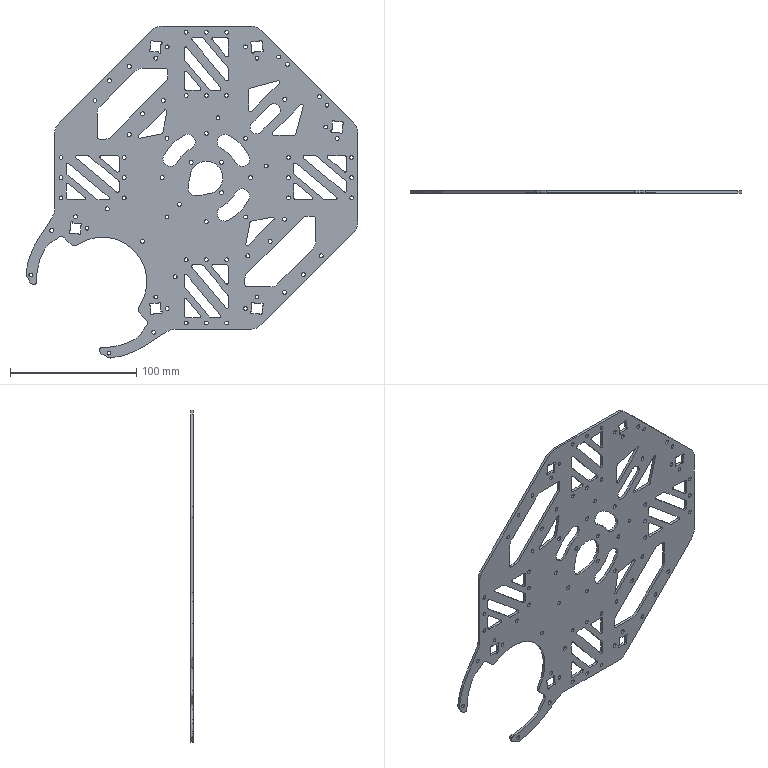Part | SolidWorks | features Fillet 7, Extrusion 1, ICE 1 | 1 solid | 443 faces | box 262.722 x 2 x 262.722 mm | volume 67464 mm3 | cylinder 317 | plane 125 | spline 1 | commonest cylinder face diameters 3 x80 3.1 x64 2.4 x56 4 x32 2 x30 24 x10